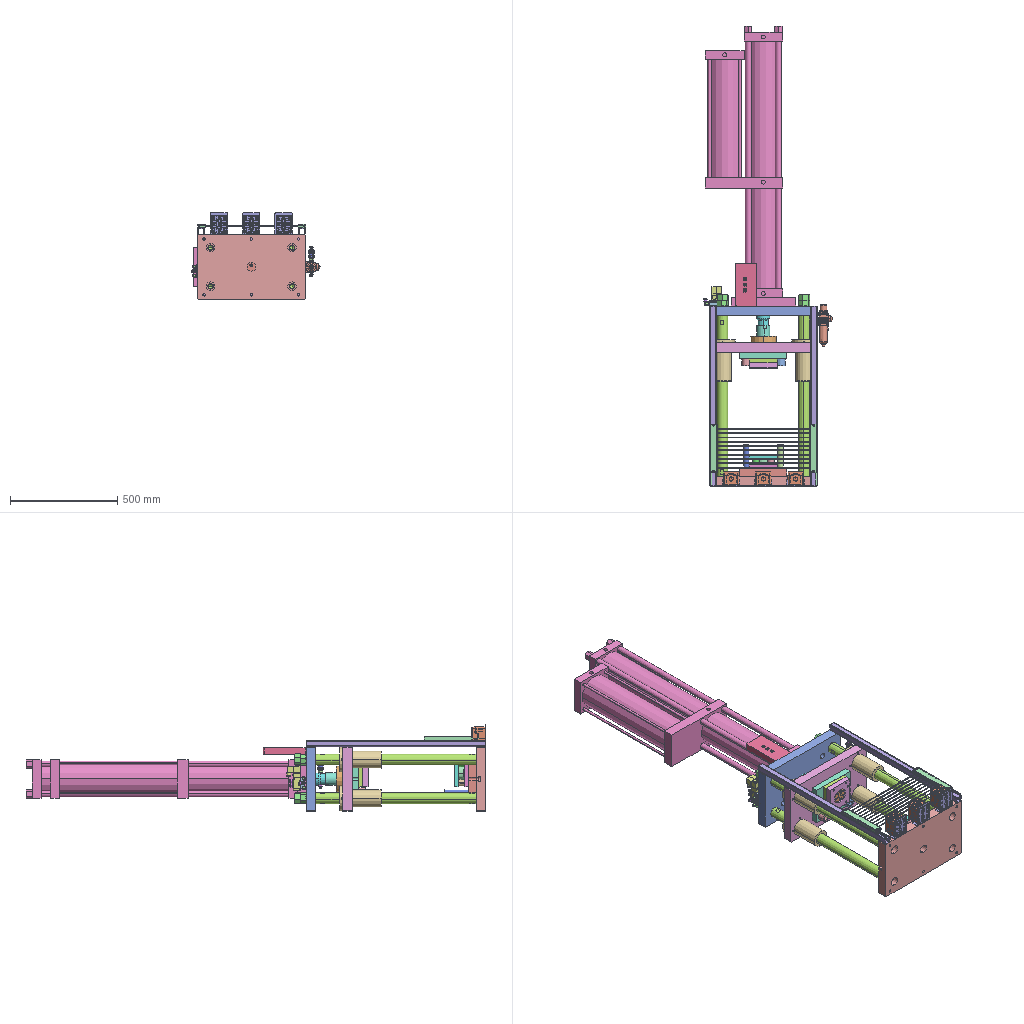Assembly | SolidWorks | 56 different items | 84 placed | box 598 x 2143 x 402 mm
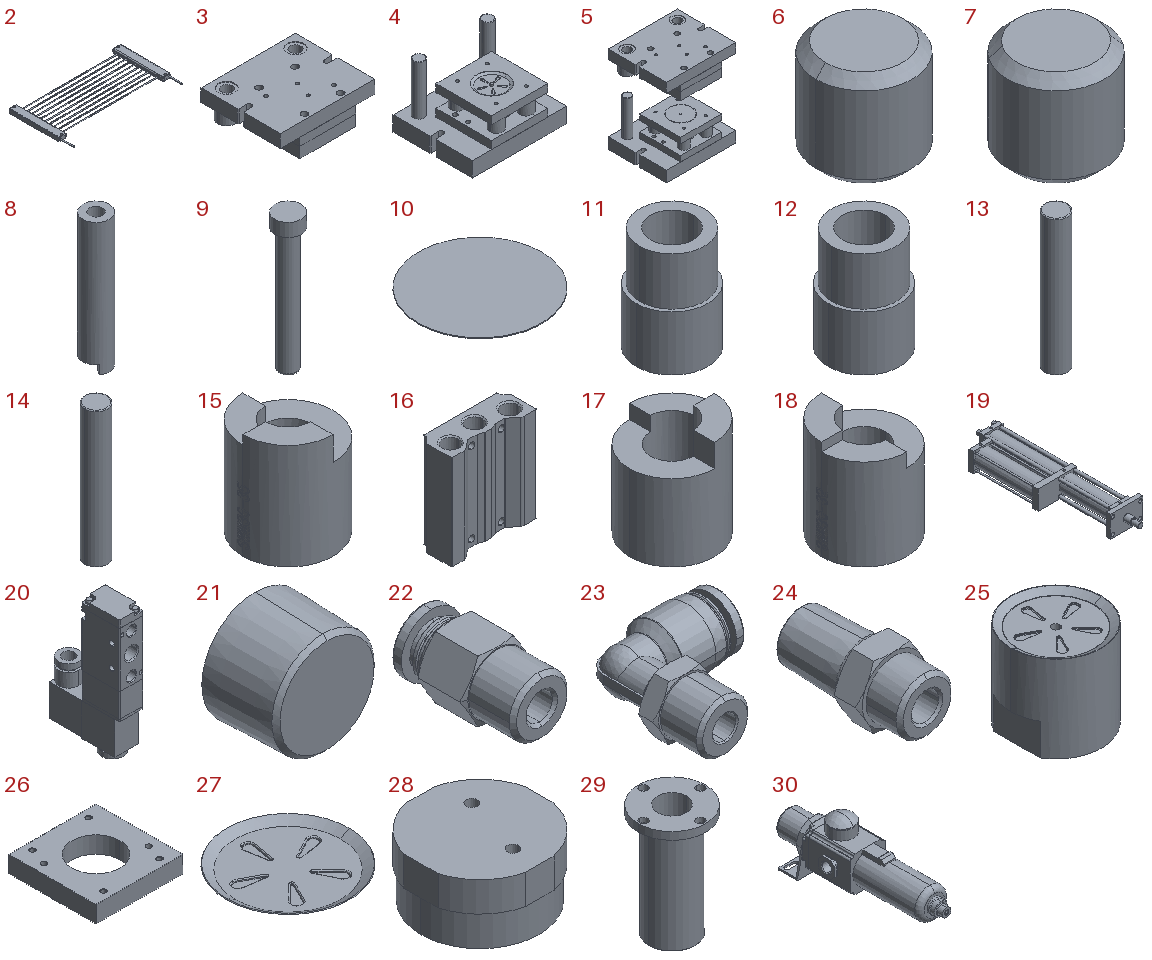Parts list (item | name | quantity | parent item | size | volume | features):
1 | (subassembly) | x1 | - | - | - | -
2 | (subassembly) | x1 | - | - | - | -
3 | (subassembly) | x1 | in 5 | 220 x 185 x 73 mm | 1914811 mm3 | -
4 | (subassembly) | x1 | in 5 | 220 x 185 x 150 mm | 2240435 mm3 | -
5 | (subassembly) | x1 | - | 220 x 185 x 276.914 mm | 4159283 mm3 | -
6 | - | x1 | in 3 | 8.005 x 8.005 x 8 mm | 387.604 mm3 | features BaseBody 1
7 | - | x1 | in 3 | 8.005 x 8.005 x 8 mm | 387.604 mm3 | features BaseBody 1
8 | - | x1 | in 3 | 6 x 6 x 30 mm | 609.259 mm3 | features BaseBody 1
9 | - | x1 | in 3 | 6 x 6 x 31 mm | 436.445 mm3 | features BaseBody 1
10 | - | x1 | in 5 | 71.5 x 71.5 x 0.5 mm | 2008 mm3 | features BaseBody 1
11 | - | x1 | in 3 | 42 x 42 x 60 mm | 46637 mm3 | features BaseBody 1
12 | - | x1 | in 3 | 42 x 42 x 60 mm | 46637 mm3 | features BaseBody 1
13 | - | x1 | in 4 | 25 x 25 x 150 mm | 73615 mm3 | features BaseBody 1
14 | - | x1 | in 4 | 25 x 25 x 150 mm | 73615 mm3 | features BaseBody 1
15 | - | x1 | in 4 | 30 x 30 x 35 mm | 16035 mm3 | features BaseBody 1
16 | - | x1 | - | 60 x 24 x 67 mm | 58558 mm3 | features BaseBody 1
17 | - | x1 | in 4 | 30 x 30 x 35 mm | 16033 mm3 | features BaseBody 1
18 | - | x1 | in 4 | 30 x 30 x 35 mm | 16033 mm3 | features BaseBody 1
19 | - | x1 | - | 420 x 1435 x 200 mm | 41260242 mm3 | features BaseBody 1, ICE 1, MoveCopyBody 1, MoveFace 1
20 | - | x2 | - | 22 x 66.8 x 117.1 mm | 99652 mm3 | features BaseBody 1
21 | - | x1 | - | 13.344 x 9 x 13.344 mm | 1017 mm3 | features BaseBody 1
22 | - | x6 | - | 16.166 x 27 x 14 mm | 2706 mm3 | features BaseBody 1
23 | - | x1 | - | - | - | features RefSurface 1
24 | - | x4 | - | - | - | features RefSurface 2
25 | - | x1 | in 4 | 71.5 x 71.5 x 68 mm | 251078 mm3 | features BaseBody 1
26 | - | x1 | in 3 | 130 x 130 x 25 mm | 315785 mm3 | features BaseBody 1
27 | - | x1 | in 5 | 70 x 70 x 4.429 mm | 2054 mm3 | features BaseBody 1
28 | - | x1 | in 3 | 72 x 72.5 x 41.7 mm | 164977 mm3 | features BaseBody 1
29 | - | x4 | - | 116 x 116 x 192 mm | 653901 mm3 | features CirPattern 1, Fillet 1, ICE 1, RevCut 1, Revolution 1
30 | - | x1 | - | 55 x 192.5 x 70.622 mm | 237290 mm3 | features BaseBody 1
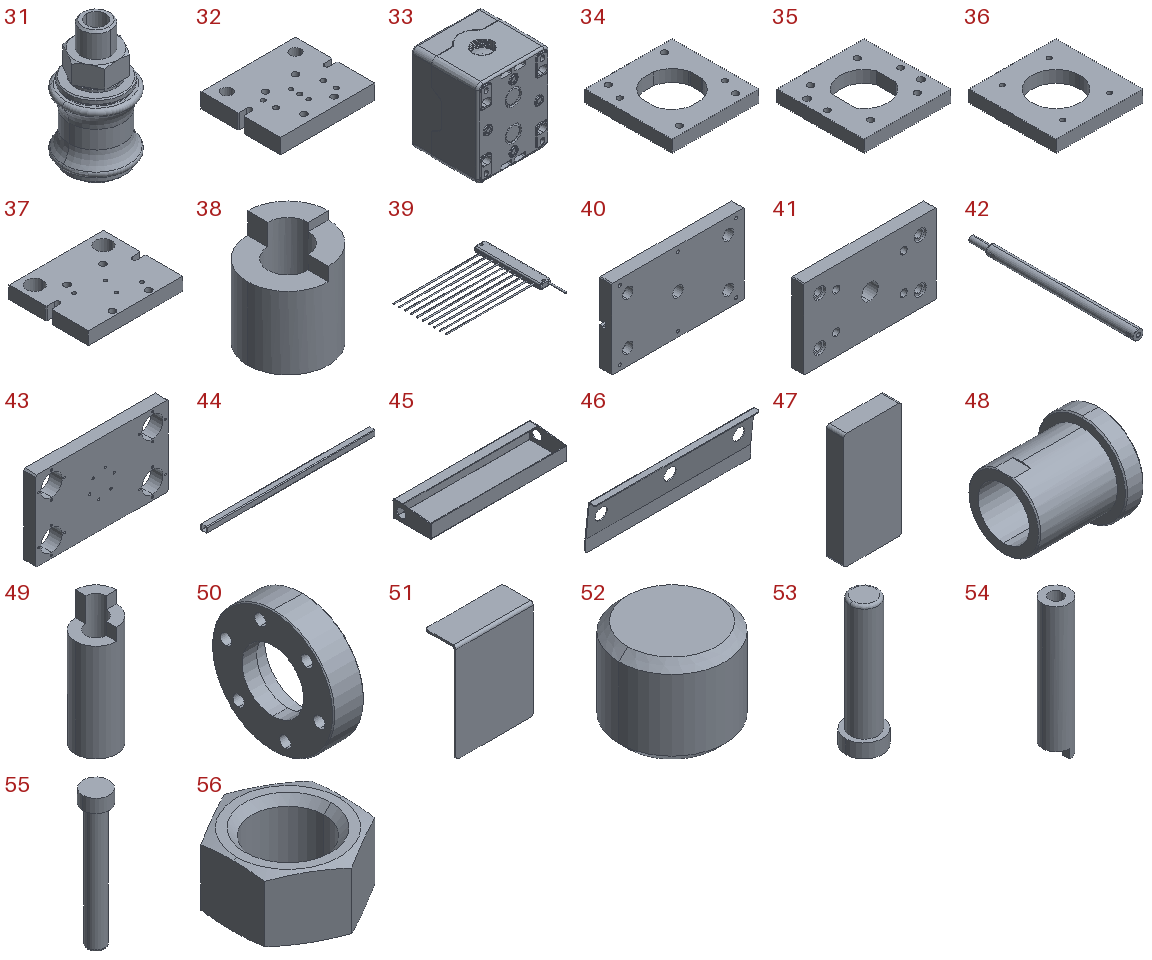31 | - | x1 | - | 30 x 30 x 58 mm | 20249 mm3 | features BaseBody 2
32 | - | x1 | in 4 | 220 x 185 x 35 mm | 1319567 mm3 | features BaseBody 1, MoveFace 1
33 | - | x3 | - | 70.742 x 66 x 85.872 mm | 117624 mm3 | features BaseBody 2
34 | - | x1 | in 3 | 130 x 130 x 18 mm | 220294 mm3 | features BaseBody 1
35 | - | x1 | in 4 | 130 x 130 x 18 mm | 225680 mm3 | features BaseBody 1
36 | - | x1 | in 4 | 130 x 130 x 18 mm | 229251 mm3 | features BaseBody 1
37 | - | x1 | in 3 | 220 x 185 x 30 mm | 1117612 mm3 | features BaseBody 1, MoveFace 1
38 | - | x1 | in 4 | 30 x 30 x 35 mm | 16035 mm3 | features BaseBody 1
39 | - | x2 | in 2 | - | - | features BaseBody 1, ExtruRefSurface 1
40 | - | x1 | - | 500 x 45 x 300 mm | 6344186 mm3 | features ICE 3, Fillet 2, HoleWzd 2, Chamfer 1, Extrusion 1, MirrorPattern 1
41 | - | x1 | - | 500 x 45 x 300 mm | 6350695 mm3 | features HoleWzd 3, ICE 2, Chamfer 1, Cut 1, Extrusion 1
42 | - | x4 | - | 50 x 853 x 50 mm | 1528965 mm3 | features ICE 5, LibraryFeature 3, Chamfer 1, Extrusion 1, HoleWzd 1
43 | - | x1 | - | 500 x 45 x 300 mm | 5801502 mm3 | features HoleWzd 2, Chamfer 1, Cut 1, Extrusion 1
44 | - | x2 | - | 838 x 30 x 30 mm | 180231 mm3 | features WeldMemberFeat 1, WeldmentFeature 1
45 | - | x1 | - | 300 x 83 x 36.5 mm | 80291 mm3 | features EdgeFlange 4, Fillet 2, CornerFeat 1, FlatPattern 1, ICE 1, SMBaseFlange 1, SheetMetal 1
46 | - | x1 | - | 300 x 18.411 x 83 mm | 40385 mm3 | features Fillet 1, FlatPattern 1, ICE 1, SMBaseFlange 1, SheetMetal 1
47 | - | x1 | - | 100 x 30 x 200 mm | 599338 mm3 | features Extrusion 1, Fillet 1, ICE 1
48 | - | x1 | - | 80 x 75 x 75 mm | 133252 mm3 | features Chamfer 1, HoleWzd 1, ICE 1, LibraryFeature 1, Revolution 1
49 | - | x1 | in 4 | 10 x 10 x 30 mm | 1546 mm3 | features BaseBody 1
50 | - | x1 | - | 30 x 120 x 120 mm | 209812 mm3 | features Chamfer 1, CirPattern 1, HoleWzd 1, Revolution 1
51 | - | x3 | - | 80 x 32 x 102 mm | 20981 mm3 | features Fillet 1, FlatPattern 1, SMBaseFlange 1, SheetMetal 1
52 | - | x1 | in 4 | 12.005 x 12.005 x 10 mm | 1096 mm3 | features BaseBody 1
53 | - | x1 | in 4 | 8 x 8 x 28 mm | 856.499 mm3 | features BaseBody 1
54 | - | x1 | in 3 | 6 x 6 x 30 mm | 609.259 mm3 | features BaseBody 1
55 | - | x1 | in 3 | 6 x 6 x 31 mm | 436.445 mm3 | features BaseBody 1
56 | - | x8 | - | 46 x 53.116 x 26.4 mm | 28471 mm3 | features Chamfer 1, Extrusion 1, ICE 1, MirrorPattern 1, RevCutThin 1
Mates (type | each side: item.copy, entity, surface, feature):
In the top assembly
Width | 40.1 face plane Boss-Extrude 1 | 40.1 face plane Boss-Extrude 1 | 41.1 face plane Boss-Extrude 1 | 41.1 face plane Boss-Extrude 1
Width | 41.1 face plane Boss-Extrude 1 | 41.1 face plane Boss-Extrude 1 | 40.1 face plane Boss-Extrude 1 | 40.1 face plane Boss-Extrude 1
Concentric | 40.1 face cylinder Cut-Extrude 1 | 42.1 face cylinder Boss-Extrude 1
Coincident | 40.1 face plane Cut-Extrude 1 | 42.1 face plane Boss-Extrude 1
Concentric | 40.1 face cylinder Cut-Extrude 1 | 42.2 face cylinder Boss-Extrude 1
Coincident | 40.1 face plane Cut-Extrude 1 | 42.2 face plane Boss-Extrude 1
Concentric | 40.1 face cylinder Cut-Extrude 1 | 42.3 face cylinder Boss-Extrude 1
Coincident | 40.1 face plane Cut-Extrude 1 | 42.3 face plane Boss-Extrude 1
Concentric | 40.1 face cylinder Cut-Extrude 1 | 42.4 face cylinder Boss-Extrude 1
Coincident | 40.1 face plane Cut-Extrude 1 | 42.4 face plane Boss-Extrude 1
Width | 43.1 face plane Boss-Extrude 1 | 43.1 face plane Boss-Extrude 1 | 40.1 face plane Boss-Extrude 1 | 40.1 face plane Boss-Extrude 1 | 2 times
Coincident | 41.1 face plane Boss-Extrude 1 | assembly face
Parallel | 41.1 face plane Boss-Extrude 1 | assembly face
Coincident | 43.1 face plane Boss-Extrude 1 | 50.1 face plane Revolve 1
Parallel | 43.1 face plane Boss-Extrude 1 | 50.1 plane
Symmetric | 43.1 face plane Boss-Extrude 1 | 43.1 face plane Boss-Extrude 1 | 50.1 plane | 2 times
Concentric | 48.1 face cylinder Revolve 1 | 50.1 face cylinder Revolve 1
Coincident | 48.1 face plane Revolve 1 | assembly face
Concentric | 50.1 face cylinder Revolve 1 | assembly face
Coincident | 48.1 face plane Revolve 1 | 50.1 face plane Revolve 1
Coincident | 16.1 face plane 200M2F | 20.1 face plane Input 1
Concentric | 16.1 face cylinder 200M2F | 20.1 face cylinder Input 1 | 2 times
Coincident | 16.1 face plane 200M2F | 20.2 face plane Input 1
Concentric | 16.1 face cylinder 200M2F | 20.2 face cylinder Input 1 | 2 times
Coincident | 41.1 face plane Boss-Extrude 1 | 16.1 face plane 200M2F | 2 times
Concentric | 16.1 face cylinder 200M2F | 24.1 face cylinder Surface-Input 7
Coincident | 16.1 face plane 200M2F | 24.1 face plane Surface-Input 7
Concentric | 16.1 face cylinder 200M2F | 24.2 face cylinder Surface-Input 7
Coincident | 16.1 face plane 200M2F | 24.2 face plane Surface-Input 7
Concentric | 16.1 face cylinder 200M2F | 24.3 face cylinder Surface-Input 7
Coincident | 16.1 face plane 200M2F | 24.3 face plane Surface-Input 7
Concentric | 16.1 face cylinder 200M2F | 24.4 face cylinder Surface-Input 7
Coincident | 16.1 face plane 200M2F | 24.4 face plane Surface-Input 7
Concentric | 20.1 face cylinder Input 1 | 22.1 face cylinder Input 1
DistanceDim | 22.1 face plane Input 1 | 20.1 face plane Input 1
Concentric | 20.1 face cylinder Input 1 | 22.2 face cylinder Input 1
DistanceDim | 22.2 face plane Input 1 | 20.1 face plane Input 1
Concentric | 20.2 face cylinder Input 1 | 22.3 face cylinder Input 1
DistanceDim | 22.3 face plane Input 1 | 20.2 face plane Input 1
Concentric | 20.2 face cylinder Input 1 | 22.4 face cylinder Input 1
DistanceDim | 22.4 face plane Input 1 | 20.2 face plane Input 1
Concentric | 16.1 face cylinder 200M2F | 23.1 face cylinder Surface-Input 10
DistanceDim | 23.1 face plane Surface-Input 10 | 16.1 face plane 200M2F
Concentric | 16.1 face cylinder 200M2F | 21.1 face cone Input 1
Coincident | 16.1 face plane 200M2F | 21.1 face plane Input 1
Coincident | 41.1 face plane Boss-Extrude 1 | 30.1 face plane GPFR20008SM
Width | 41.1 face plane Boss-Extrude 1 | 41.1 face plane Boss-Extrude 1 | 30.1 face plane GPFR20008SM | 30.1 face plane GPFR20008SM
DistanceDim | 41.1 face plane Boss-Extrude 1 | 30.1 face plane GPFR20008SM
Concentric | 30.1 face cylinder GPFR20008SM | 31.1 face cylinder HSV08 Body-1-solid1
DistanceDim | 31.1 face plane HSV08 Body-1-solid1 | 30.1 face plane GPFR20008SM
Concentric | 31.1 face cylinder HSV08 Body-1-solid1 | 22.5 face cylinder Input 1
DistanceDim | 22.5 face plane Input 1 | 31.1 face plane HSV08 Body-1-solid1
Concentric | 30.1 face cylinder GPFR20008SM | 22.6 face cylinder Input 1
Coincident | 30.1 face plane GPFR20008SM | 22.6 face plane Input 1
Coincident | 41.1 face plane Boss-Extrude 1 | 42.1 face plane Boss-Extrude 1
Concentric | 42.1 face cylinder Boss-Extrude 2 | 56.1 face cylinder Cut-Extrude1
Coincident | 41.1 face plane Boss-Extrude 1 | 56.1 face plane Boss-Extrude1
Concentric | 42.1 face cylinder Boss-Extrude 2 | 56.2 face cylinder Cut-Extrude1
Coincident | 56.1 face plane Boss-Extrude1 | 56.2 face plane Boss-Extrude1
Concentric | 42.2 face cylinder Boss-Extrude 2 | 56.3 face cylinder Cut-Extrude1
Coincident | 41.1 face plane Boss-Extrude 1 | 56.3 face plane Boss-Extrude1
Concentric | 42.2 face cylinder Boss-Extrude 2 | 56.4 face cylinder Cut-Extrude1
Coincident | 56.3 face plane Boss-Extrude1 | 56.4 face plane Boss-Extrude1
Concentric | 42.3 face cylinder Boss-Extrude 2 | 56.5 face cylinder Cut-Extrude1
Coincident | 41.1 face plane Boss-Extrude 1 | 56.5 face plane Boss-Extrude1
Concentric | 42.3 face cylinder Boss-Extrude 2 | 56.6 face cylinder Cut-Extrude1
Coincident | 56.5 face plane Boss-Extrude1 | 56.6 face plane Boss-Extrude1
Concentric | 42.4 face cylinder Boss-Extrude 2 | 56.7 face cylinder Cut-Extrude1
Coincident | 41.1 face plane Boss-Extrude 1 | 56.7 face plane Boss-Extrude1
Concentric | 42.4 face cylinder Boss-Extrude 2 | 56.8 face cylinder Cut-Extrude1
Coincident | 56.7 face plane Boss-Extrude1 | 56.8 face plane Boss-Extrude1
Coincident | 40.1 face plane Boss-Extrude 1 | 44.1 face plane Unnamed 30×2(1) | 3 times
Coincident | 40.1 face plane Boss-Extrude 1 | 44.2 face plane Unnamed 30×2(1) | 3 times
Coincident | 39.1 face plane Input 1 | 44.1 face plane Unnamed 30×2(1)
Width | 39.1 face plane Input 1 | 39.1 face plane Input 1 | 44.1 face plane Unnamed 30×2(1) | 44.1 face plane Unnamed 30×2(1)
Coincident | 40.1 face plane Boss-Extrude 1 | 45.1 face | 2 times
Coincident | 45.1 face | 46.1 face | 2 times
Width | 45.1 face | 45.1 face | 46.1 face | 46.1 face
Width | 40.1 face plane Boss-Extrude 1 | 40.1 face plane Boss-Extrude 1 | 45.1 face | 45.1 face
Coincident | 41.1 face plane Boss-Extrude 1 | 47.1 face plane Boss-Extrude 1
DistanceDim | 47.1 face plane Boss-Extrude 1 | 41.1 face plane Boss-Extrude 1 | 2 times
Coincident | 41.1 face plane Boss-Extrude 1 | 19.1 face plane Input 1
Width | 19.1 face plane Input 1 | 19.1 face plane Input 1 | 41.1 face plane Boss-Extrude 1 | 41.1 face plane Boss-Extrude 1 | 2 times
DistanceDim | 16.1 face plane 200M2F | 41.1 face plane Boss-Extrude 1
Concentric | 42.2 face cylinder Boss-Extrude 1 | 29.1 face cylinder Revolve 1
Coincident | 43.1 face plane Boss-Extrude 1 | 29.1 face plane Boss-Extrude 1
Parallel | 43.1 face plane Boss-Extrude 1 | 29.1 plane
Concentric | 42.1 face cylinder Boss-Extrude 1 | 29.2 face cylinder Revolve 1
Coincident | 43.1 face plane Boss-Extrude 1 | 29.2 face plane Boss-Extrude 1
Parallel | 43.1 face plane Boss-Extrude 1 | 29.2 plane
Concentric | 42.4 face cylinder Boss-Extrude 1 | 29.3 face cylinder Revolve 1
Coincident | 43.1 face plane Boss-Extrude 1 | 29.3 face plane Boss-Extrude 1
Parallel | 43.1 face plane Boss-Extrude 1 | 29.3 plane
Concentric | 42.3 face cylinder Boss-Extrude 1 | 29.4 face cylinder Revolve 1
Coincident | 43.1 face plane Boss-Extrude 1 | 29.4 face plane Boss-Extrude 1
Parallel | 43.1 face plane Boss-Extrude 1 | 29.4 plane
DistanceDim | 48.1 face plane Revolve 1 | 19.1 face plane Input 1
Coincident | 40.1 face plane Boss-Extrude 1 | assembly face
Width | assembly face | assembly face | 40.1 face plane Boss-Extrude 1 | 40.1 face plane Boss-Extrude 1 | 2 times
Coincident | 40.1 face plane Boss-Extrude 1 | 32.1 face plane Input 1
Width | 32.1 face plane Input 1 | 32.1 face plane Input 1 | 40.1 face plane Boss-Extrude 1 | 40.1 face plane Boss-Extrude 1 | 2 times
Coincident | 43.1 face plane Boss-Extrude 1 | 37.1 face plane Input 1
Coincident | 40.1 face plane Boss-Extrude 1 | 51.1 face plane Base-Flange 1 | 2 times
Coincident | 33.1 face plane Input 2 | 51.1 face plane Base-Flange 1
Width | 33.1 face plane Input 2 | 33.1 face plane Input 2 | 51.1 face plane Base-Flange 1 | 51.1 face plane Base-Flange 1
DistanceDim | 33.1 edge | 51.1 face plane Base-Flange 1
Width | 40.1 face plane Boss-Extrude 1 | 40.1 face plane Boss-Extrude 1 | 51.2 face plane Base-Flange 1 | 51.1 face plane Base-Flange 1
In subassembly 2
Symmetric | 39.2 face plane Input 1 | 39.2 face plane Input 1 | 2.1 plane | 2 times
Symmetric | 39.3 face plane Input 1 | 39.3 face plane Input 1 | 2.1 plane
Coincident | 39.2 face plane Input 1 | 39.3 face plane Input 1
DistanceDim | 39.2 edge | 39.3 face plane Input 1
Symmetric | 39.2 face plane Input 1 | 39.3 face plane Input 1 | 2.1 plane
In subassembly 5
Concentric | 11.1 face cylinder Input 1 | 13.1 face cylinder Input 1
Concentric | 12.1 face cylinder Input 1 | 14.1 face cylinder Input 1